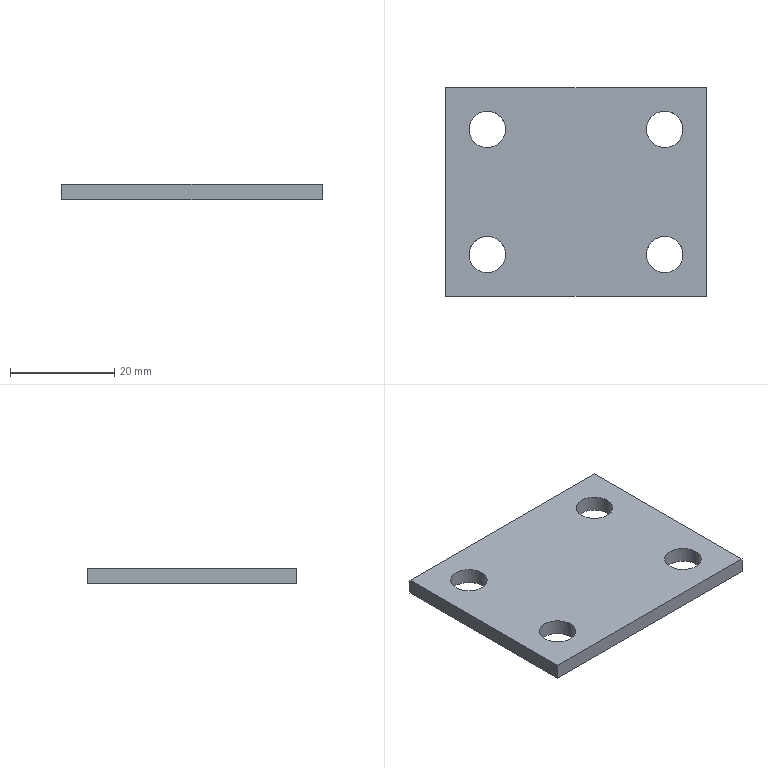Part | STEP file | Positioning_id2102_x_t | 1 solid | 14 faces | box 50 x 40 x 3 mm | volume 5538 mm3 | cylinder 8 | plane 6 | commonest cylinder face diameters 7 x8
STEP:
#1=CARTESIAN_POINT('',(0.,0.,0.));
#2=DIRECTION('',(0.,0.,1.));
#3=DIRECTION('',(1.,0.,0.));
#4=AXIS2_PLACEMENT_3D('',#1,#2,#3);
#5=CARTESIAN_POINT('',(-816.502,12.,379.5));
#6=VERTEX_POINT('',#5);
#7=CARTESIAN_POINT('',(-823.502,12.,379.5));
#8=VERTEX_POINT('',#7);
#9=CARTESIAN_POINT('',(-820.002,12.,379.5));
#10=DIRECTION('',(0.,0.,-1.));
#11=DIRECTION('',(1.,0.,0.));
#12=AXIS2_PLACEMENT_3D('',#9,#10,#11);
#13=CIRCLE('',#12,3.5);
#14=CARTESIAN_POINT('',(-773.002,-20.,379.5));
#15=DIRECTION('',(0.,0.,-1.));
#16=DIRECTION('',(-1.,0.,0.));
#17=AXIS2_PLACEMENT_3D('',#14,#15,#16);
#18=PLANE('',#17);
#19=CARTESIAN_POINT('',(47.,32.));
#20=DIRECTION('',(-1.,0.));
#21=AXIS2_PLACEMENT_2D('',#19,#20);
#22=CIRCLE('',#21,3.5);
#23=(GEOMETRIC_REPRESENTATION_CONTEXT(2)PARAMETRIC_REPRESENTATION_CONTEXT()REPRESENTATION_CONTEXT('',''));
#24=DEFINITIONAL_REPRESENTATION('',(#22),#23);
#25=PCURVE('',#18,#24);
#26=CARTESIAN_POINT('',(-820.002,12.,392.15));
#27=DIRECTION('',(0.,0.,1.));
#28=DIRECTION('',(-1.,0.,0.));
#29=AXIS2_PLACEMENT_3D('',#26,#27,#28);
#30=CYLINDRICAL_SURFACE('',#29,3.5);
#31=CARTESIAN_POINT('',(3.142,-12.65));
#32=DIRECTION('',(-1.,0.));
#33=VECTOR('',#32,1.);
#34=LINE('',#31,#33);
#35=(GEOMETRIC_REPRESENTATION_CONTEXT(2)PARAMETRIC_REPRESENTATION_CONTEXT()REPRESENTATION_CONTEXT('',''));
#36=DEFINITIONAL_REPRESENTATION('',(#34),#35);
#37=PCURVE('',#30,#36);
#38=SURFACE_CURVE('',#13,(#25,#37),.PCURVE_S1.);
#39=EDGE_CURVE('',#6,#8,#38,.T.);
#40=ORIENTED_EDGE('',*,*,#39,.T.);
#41=CARTESIAN_POINT('',(-820.002,15.5,379.5));
#42=VERTEX_POINT('',#41);
#43=CARTESIAN_POINT('',(-820.002,12.,379.5));
#44=DIRECTION('',(0.,0.,-1.));
#45=DIRECTION('',(-1.,0.,0.));
#46=AXIS2_PLACEMENT_3D('',#43,#44,#45);
#47=CIRCLE('',#46,3.5);
#48=CARTESIAN_POINT('',(47.,32.));
#49=DIRECTION('',(1.,0.));
#50=AXIS2_PLACEMENT_2D('',#48,#49);
#51=CIRCLE('',#50,3.5);
#52=(GEOMETRIC_REPRESENTATION_CONTEXT(2)PARAMETRIC_REPRESENTATION_CONTEXT()REPRESENTATION_CONTEXT('',''));
#53=DEFINITIONAL_REPRESENTATION('',(#51),#52);
#54=PCURVE('',#18,#53);
#55=CARTESIAN_POINT('',(-820.002,12.,392.15));
#56=DIRECTION('',(0.,0.,1.));
#57=DIRECTION('',(-1.,0.,0.));
#58=AXIS2_PLACEMENT_3D('',#55,#56,#57);
#59=CYLINDRICAL_SURFACE('',#58,3.5);
#60=CARTESIAN_POINT('',(6.283,-12.65));
#61=DIRECTION('',(-1.,0.));
#62=VECTOR('',#61,1.);
#63=LINE('',#60,#62);
#64=(GEOMETRIC_REPRESENTATION_CONTEXT(2)PARAMETRIC_REPRESENTATION_CONTEXT()REPRESENTATION_CONTEXT('',''));
#65=DEFINITIONAL_REPRESENTATION('',(#63),#64);
#66=PCURVE('',#59,#65);
#67=SURFACE_CURVE('',#47,(#54,#66),.PCURVE_S1.);
#68=EDGE_CURVE('',#8,#42,#67,.T.);
#69=ORIENTED_EDGE('',*,*,#68,.T.);
#70=CARTESIAN_POINT('',(-820.002,12.,379.5));
#71=DIRECTION('',(0.,0.,-1.));
#72=DIRECTION('',(0.,1.,0.));
#73=AXIS2_PLACEMENT_3D('',#70,#71,#72);
#74=CIRCLE('',#73,3.5);
#75=CARTESIAN_POINT('',(47.,32.));
#76=DIRECTION('',(0.,1.));
#77=AXIS2_PLACEMENT_2D('',#75,#76);
#78=CIRCLE('',#77,3.5);
#79=(GEOMETRIC_REPRESENTATION_CONTEXT(2)PARAMETRIC_REPRESENTATION_CONTEXT()REPRESENTATION_CONTEXT('',''));
#80=DEFINITIONAL_REPRESENTATION('',(#78),#79);
#81=PCURVE('',#18,#80);
#82=CARTESIAN_POINT('',(4.712,-12.65));
#83=DIRECTION('',(-1.,0.));
#84=VECTOR('',#83,1.);
#85=LINE('',#82,#84);
#86=(GEOMETRIC_REPRESENTATION_CONTEXT(2)PARAMETRIC_REPRESENTATION_CONTEXT()REPRESENTATION_CONTEXT('',''));
#87=DEFINITIONAL_REPRESENTATION('',(#85),#86);
#88=PCURVE('',#59,#87);
#89=SURFACE_CURVE('',#74,(#81,#88),.PCURVE_S1.);
#90=EDGE_CURVE('',#42,#6,#89,.T.);
#91=ORIENTED_EDGE('',*,*,#90,.T.);
#92=EDGE_LOOP('',(#40,#69,#91));
#93=FACE_BOUND('',#92,.T.);
#94=CARTESIAN_POINT('',(-782.502,-12.,379.5));
#95=VERTEX_POINT('',#94);
#96=CARTESIAN_POINT('',(-789.502,-12.,379.5));
#97=VERTEX_POINT('',#96);
#98=CARTESIAN_POINT('',(-786.002,-12.,379.5));
#99=DIRECTION('',(0.,0.,-1.));
#100=DIRECTION('',(1.,0.,0.));
#101=AXIS2_PLACEMENT_3D('',#98,#99,#100);
#102=CIRCLE('',#101,3.5);
#103=CARTESIAN_POINT('',(13.,8.));
#104=DIRECTION('',(-1.,0.));
#105=AXIS2_PLACEMENT_2D('',#103,#104);
#106=CIRCLE('',#105,3.5);
#107=(GEOMETRIC_REPRESENTATION_CONTEXT(2)PARAMETRIC_REPRESENTATION_CONTEXT()REPRESENTATION_CONTEXT('',''));
#108=DEFINITIONAL_REPRESENTATION('',(#106),#107);
#109=PCURVE('',#18,#108);
#110=CARTESIAN_POINT('',(-786.002,-12.,392.15));
#111=DIRECTION('',(0.,0.,1.));
#112=DIRECTION('',(-1.,0.,0.));
#113=AXIS2_PLACEMENT_3D('',#110,#111,#112);
#114=CYLINDRICAL_SURFACE('',#113,3.5);
#115=CARTESIAN_POINT('',(3.142,-12.65));
#116=DIRECTION('',(-1.,0.));
#117=VECTOR('',#116,1.);
#118=LINE('',#115,#117);
#119=(GEOMETRIC_REPRESENTATION_CONTEXT(2)PARAMETRIC_REPRESENTATION_CONTEXT()REPRESENTATION_CONTEXT('',''));
#120=DEFINITIONAL_REPRESENTATION('',(#118),#119);
#121=PCURVE('',#114,#120);
#122=SURFACE_CURVE('',#102,(#109,#121),.PCURVE_S1.);
#123=EDGE_CURVE('',#95,#97,#122,.T.);
#124=ORIENTED_EDGE('',*,*,#123,.T.);
#125=CARTESIAN_POINT('',(-786.002,-8.5,379.5));
#126=VERTEX_POINT('',#125);
#127=CARTESIAN_POINT('',(-786.002,-12.,379.5));
#128=DIRECTION('',(0.,0.,-1.));
#129=DIRECTION('',(-1.,0.,0.));
#130=AXIS2_PLACEMENT_3D('',#127,#128,#129);
#131=CIRCLE('',#130,3.5);
#132=CARTESIAN_POINT('',(13.,8.));
#133=DIRECTION('',(1.,0.));
#134=AXIS2_PLACEMENT_2D('',#132,#133);
#135=CIRCLE('',#134,3.5);
#136=(GEOMETRIC_REPRESENTATION_CONTEXT(2)PARAMETRIC_REPRESENTATION_CONTEXT()REPRESENTATION_CONTEXT('',''));
#137=DEFINITIONAL_REPRESENTATION('',(#135),#136);
#138=PCURVE('',#18,#137);
#139=CARTESIAN_POINT('',(-786.002,-12.,392.15));
#140=DIRECTION('',(0.,0.,1.));
#141=DIRECTION('',(-1.,0.,0.));
#142=AXIS2_PLACEMENT_3D('',#139,#140,#141);
#143=CYLINDRICAL_SURFACE('',#142,3.5);
#144=CARTESIAN_POINT('',(6.283,-12.65));
#145=DIRECTION('',(-1.,0.));
#146=VECTOR('',#145,1.);
#147=LINE('',#144,#146);
#148=(GEOMETRIC_REPRESENTATION_CONTEXT(2)PARAMETRIC_REPRESENTATION_CONTEXT()REPRESENTATION_CONTEXT('',''));
#149=DEFINITIONAL_REPRESENTATION('',(#147),#148);
#150=PCURVE('',#143,#149);
#151=SURFACE_CURVE('',#131,(#138,#150),.PCURVE_S1.);
#152=EDGE_CURVE('',#97,#126,#151,.T.);
#153=ORIENTED_EDGE('',*,*,#152,.T.);
#154=CARTESIAN_POINT('',(-786.002,-12.,379.5));
#155=DIRECTION('',(0.,0.,-1.));
#156=DIRECTION('',(0.,1.,0.));
#157=AXIS2_PLACEMENT_3D('',#154,#155,#156);
#158=CIRCLE('',#157,3.5);
#159=CARTESIAN_POINT('',(13.,8.));
#160=DIRECTION('',(0.,1.));
#161=AXIS2_PLACEMENT_2D('',#159,#160);
#162=CIRCLE('',#161,3.5);
#163=(GEOMETRIC_REPRESENTATION_CONTEXT(2)PARAMETRIC_REPRESENTATION_CONTEXT()REPRESENTATION_CONTEXT('',''));
#164=DEFINITIONAL_REPRESENTATION('',(#162),#163);
#165=PCURVE('',#18,#164);
#166=CARTESIAN_POINT('',(4.712,-12.65));
#167=DIRECTION('',(-1.,0.));
#168=VECTOR('',#167,1.);
#169=LINE('',#166,#168);
#170=(GEOMETRIC_REPRESENTATION_CONTEXT(2)PARAMETRIC_REPRESENTATION_CONTEXT()REPRESENTATION_CONTEXT('',''));
#171=DEFINITIONAL_REPRESENTATION('',(#169),#170);
#172=PCURVE('',#143,#171);
#173=SURFACE_CURVE('',#158,(#165,#172),.PCURVE_S1.);
#174=EDGE_CURVE('',#126,#95,#173,.T.);
#175=ORIENTED_EDGE('',*,*,#174,.T.);
#176=EDGE_LOOP('',(#124,#153,#175));
#177=FACE_BOUND('',#176,.T.);
#178=CARTESIAN_POINT('',(-782.502,12.,379.5));
#179=VERTEX_POINT('',#178);
#180=CARTESIAN_POINT('',(-789.502,12.,379.5));
#181=VERTEX_POINT('',#180);
#182=CARTESIAN_POINT('',(-786.002,12.,379.5));
#183=DIRECTION('',(0.,0.,-1.));
#184=DIRECTION('',(1.,0.,0.));
#185=AXIS2_PLACEMENT_3D('',#182,#183,#184);
#186=CIRCLE('',#185,3.5);
#187=CARTESIAN_POINT('',(13.,32.));
#188=DIRECTION('',(-1.,0.));
#189=AXIS2_PLACEMENT_2D('',#187,#188);
#190=CIRCLE('',#189,3.5);
#191=(GEOMETRIC_REPRESENTATION_CONTEXT(2)PARAMETRIC_REPRESENTATION_CONTEXT()REPRESENTATION_CONTEXT('',''));
#192=DEFINITIONAL_REPRESENTATION('',(#190),#191);
#193=PCURVE('',#18,#192);
#194=CARTESIAN_POINT('',(-786.002,12.,392.15));
#195=DIRECTION('',(0.,0.,1.));
#196=DIRECTION('',(-1.,0.,0.));
#197=AXIS2_PLACEMENT_3D('',#194,#195,#196);
#198=CYLINDRICAL_SURFACE('',#197,3.5);
#199=CARTESIAN_POINT('',(3.142,-12.65));
#200=DIRECTION('',(-1.,0.));
#201=VECTOR('',#200,1.);
#202=LINE('',#199,#201);
#203=(GEOMETRIC_REPRESENTATION_CONTEXT(2)PARAMETRIC_REPRESENTATION_CONTEXT()REPRESENTATION_CONTEXT('',''));
#204=DEFINITIONAL_REPRESENTATION('',(#202),#203);
#205=PCURVE('',#198,#204);
#206=SURFACE_CURVE('',#186,(#193,#205),.PCURVE_S1.);
#207=EDGE_CURVE('',#179,#181,#206,.T.);
#208=ORIENTED_EDGE('',*,*,#207,.T.);
#209=CARTESIAN_POINT('',(-786.002,15.5,379.5));
#210=VERTEX_POINT('',#209);
#211=CARTESIAN_POINT('',(-786.002,12.,379.5));
#212=DIRECTION('',(0.,0.,-1.));
#213=DIRECTION('',(-1.,0.,0.));
#214=AXIS2_PLACEMENT_3D('',#211,#212,#213);
#215=CIRCLE('',#214,3.5);
#216=CARTESIAN_POINT('',(13.,32.));
#217=DIRECTION('',(1.,0.));
#218=AXIS2_PLACEMENT_2D('',#216,#217);
#219=CIRCLE('',#218,3.5);
#220=(GEOMETRIC_REPRESENTATION_CONTEXT(2)PARAMETRIC_REPRESENTATION_CONTEXT()REPRESENTATION_CONTEXT('',''));
#221=DEFINITIONAL_REPRESENTATION('',(#219),#220);
#222=PCURVE('',#18,#221);
#223=CARTESIAN_POINT('',(-786.002,12.,392.15));
#224=DIRECTION('',(0.,0.,1.));
#225=DIRECTION('',(-1.,0.,0.));
#226=AXIS2_PLACEMENT_3D('',#223,#224,#225);
#227=CYLINDRICAL_SURFACE('',#226,3.5);
#228=CARTESIAN_POINT('',(6.283,-12.65));
#229=DIRECTION('',(-1.,0.));
#230=VECTOR('',#229,1.);
#231=LINE('',#228,#230);
#232=(GEOMETRIC_REPRESENTATION_CONTEXT(2)PARAMETRIC_REPRESENTATION_CONTEXT()REPRESENTATION_CONTEXT('',''));
#233=DEFINITIONAL_REPRESENTATION('',(#231),#232);
#234=PCURVE('',#227,#233);
#235=SURFACE_CURVE('',#215,(#222,#234),.PCURVE_S1.);
#236=EDGE_CURVE('',#181,#210,#235,.T.);
#237=ORIENTED_EDGE('',*,*,#236,.T.);
#238=CARTESIAN_POINT('',(-786.002,12.,379.5));
#239=DIRECTION('',(0.,0.,-1.));
#240=DIRECTION('',(0.,1.,0.));
#241=AXIS2_PLACEMENT_3D('',#238,#239,#240);
#242=CIRCLE('',#241,3.5);
#243=CARTESIAN_POINT('',(13.,32.));
#244=DIRECTION('',(0.,1.));
#245=AXIS2_PLACEMENT_2D('',#243,#244);
#246=CIRCLE('',#245,3.5);
#247=(GEOMETRIC_REPRESENTATION_CONTEXT(2)PARAMETRIC_REPRESENTATION_CONTEXT()REPRESENTATION_CONTEXT('',''));
#248=DEFINITIONAL_REPRESENTATION('',(#246),#247);
#249=PCURVE('',#18,#248);
#250=CARTESIAN_POINT('',(4.712,-12.65));
#251=DIRECTION('',(-1.,0.));
#252=VECTOR('',#251,1.);
#253=LINE('',#250,#252);
#254=(GEOMETRIC_REPRESENTATION_CONTEXT(2)PARAMETRIC_REPRESENTATION_CONTEXT()REPRESENTATION_CONTEXT('',''));
#255=DEFINITIONAL_REPRESENTATION('',(#253),#254);
#256=PCURVE('',#227,#255);
#257=SURFACE_CURVE('',#242,(#249,#256),.PCURVE_S1.);
#258=EDGE_CURVE('',#210,#179,#257,.T.);
#259=ORIENTED_EDGE('',*,*,#258,.T.);
#260=EDGE_LOOP('',(#208,#237,#259));
#261=FACE_BOUND('',#260,.T.);
#262=CARTESIAN_POINT('',(-816.502,-12.,379.5));
#263=VERTEX_POINT('',#262);
#264=CARTESIAN_POINT('',(-823.502,-12.,379.5));
#265=VERTEX_POINT('',#264);
#266=CARTESIAN_POINT('',(-820.002,-12.,379.5));
#267=DIRECTION('',(0.,0.,-1.));
#268=DIRECTION('',(1.,0.,0.));
#269=AXIS2_PLACEMENT_3D('',#266,#267,#268);
#270=CIRCLE('',#269,3.5);
#271=CARTESIAN_POINT('',(47.,8.));
#272=DIRECTION('',(-1.,0.));
#273=AXIS2_PLACEMENT_2D('',#271,#272);
#274=CIRCLE('',#273,3.5);
#275=(GEOMETRIC_REPRESENTATION_CONTEXT(2)PARAMETRIC_REPRESENTATION_CONTEXT()REPRESENTATION_CONTEXT('',''));
#276=DEFINITIONAL_REPRESENTATION('',(#274),#275);
#277=PCURVE('',#18,#276);
#278=CARTESIAN_POINT('',(-820.002,-12.,392.15));
#279=DIRECTION('',(0.,0.,1.));
#280=DIRECTION('',(-1.,0.,0.));
#281=AXIS2_PLACEMENT_3D('',#278,#279,#280);
#282=CYLINDRICAL_SURFACE('',#281,3.5);
#283=CARTESIAN_POINT('',(3.142,-12.65));
#284=DIRECTION('',(-1.,0.));
#285=VECTOR('',#284,1.);
#286=LINE('',#283,#285);
#287=(GEOMETRIC_REPRESENTATION_CONTEXT(2)PARAMETRIC_REPRESENTATION_CONTEXT()REPRESENTATION_CONTEXT('',''));
#288=DEFINITIONAL_REPRESENTATION('',(#286),#287);
#289=PCURVE('',#282,#288);
#290=SURFACE_CURVE('',#270,(#277,#289),.PCURVE_S1.);
#291=EDGE_CURVE('',#263,#265,#290,.T.);
#292=ORIENTED_EDGE('',*,*,#291,.T.);
#293=CARTESIAN_POINT('',(-820.002,-8.5,379.5));
#294=VERTEX_POINT('',#293);
#295=CARTESIAN_POINT('',(-820.002,-12.,379.5));
#296=DIRECTION('',(0.,0.,-1.));
#297=DIRECTION('',(-1.,0.,0.));
#298=AXIS2_PLACEMENT_3D('',#295,#296,#297);
#299=CIRCLE('',#298,3.5);
#300=CARTESIAN_POINT('',(47.,8.));
#301=DIRECTION('',(1.,0.));
#302=AXIS2_PLACEMENT_2D('',#300,#301);
#303=CIRCLE('',#302,3.5);
#304=(GEOMETRIC_REPRESENTATION_CONTEXT(2)PARAMETRIC_REPRESENTATION_CONTEXT()REPRESENTATION_CONTEXT('',''));
#305=DEFINITIONAL_REPRESENTATION('',(#303),#304);
#306=PCURVE('',#18,#305);
#307=CARTESIAN_POINT('',(-820.002,-12.,392.15));
#308=DIRECTION('',(0.,0.,1.));
#309=DIRECTION('',(-1.,0.,0.));
#310=AXIS2_PLACEMENT_3D('',#307,#308,#309);
#311=CYLINDRICAL_SURFACE('',#310,3.5);
#312=CARTESIAN_POINT('',(6.283,-12.65));
#313=DIRECTION('',(-1.,0.));
#314=VECTOR('',#313,1.);
#315=LINE('',#312,#314);
#316=(GEOMETRIC_REPRESENTATION_CONTEXT(2)PARAMETRIC_REPRESENTATION_CONTEXT()REPRESENTATION_CONTEXT('',''));
#317=DEFINITIONAL_REPRESENTATION('',(#315),#316);
#318=PCURVE('',#311,#317);
#319=SURFACE_CURVE('',#299,(#306,#318),.PCURVE_S1.);
#320=EDGE_CURVE('',#265,#294,#319,.T.);
#321=ORIENTED_EDGE('',*,*,#320,.T.);
#322=CARTESIAN_POINT('',(-820.002,-12.,379.5));
#323=DIRECTION('',(0.,0.,-1.));
#324=DIRECTION('',(0.,1.,0.));
#325=AXIS2_PLACEMENT_3D('',#322,#323,#324);
#326=CIRCLE('',#325,3.5);
#327=CARTESIAN_POINT('',(47.,8.));
#328=DIRECTION('',(0.,1.));
#329=AXIS2_PLACEMENT_2D('',#327,#328);
#330=CIRCLE('',#329,3.5);
#331=(GEOMETRIC_REPRESENTATION_CONTEXT(2)PARAMETRIC_REPRESENTATION_CONTEXT()REPRESENTATION_CONTEXT('',''));
#332=DEFINITIONAL_REPRESENTATION('',(#330),#331);
#333=PCURVE('',#18,#332);
#334=CARTESIAN_POINT('',(4.712,-12.65));
#335=DIRECTION('',(-1.,0.));
#336=VECTOR('',#335,1.);
#337=LINE('',#334,#336);
#338=(GEOMETRIC_REPRESENTATION_CONTEXT(2)PARAMETRIC_REPRESENTATION_CONTEXT()REPRESENTATION_CONTEXT('',''));
#339=DEFINITIONAL_REPRESENTATION('',(#337),#338);
#340=PCURVE('',#311,#339);
#341=SURFACE_CURVE('',#326,(#333,#340),.PCURVE_S1.);
#342=EDGE_CURVE('',#294,#263,#341,.T.);
#343=ORIENTED_EDGE('',*,*,#342,.T.);
#344=EDGE_LOOP('',(#292,#321,#343));
#345=FACE_BOUND('',#344,.T.);
#346=CARTESIAN_POINT('',(-828.002,20.,379.5));
#347=VERTEX_POINT('',#346);
#348=CARTESIAN_POINT('',(-778.002,20.,379.5));
#349=VERTEX_POINT('',#348);
#350=CARTESIAN_POINT('',(-828.002,20.,379.5));
#351=DIRECTION('',(1.,0.,0.));
#352=VECTOR('',#351,1.);
#353=LINE('',#350,#352);
#354=CARTESIAN_POINT('',(55.,40.));
#355=DIRECTION('',(-1.,0.));
#356=VECTOR('',#355,1.);
#357=LINE('',#354,#356);
#358=(GEOMETRIC_REPRESENTATION_CONTEXT(2)PARAMETRIC_REPRESENTATION_CONTEXT()REPRESENTATION_CONTEXT('',''));
#359=DEFINITIONAL_REPRESENTATION('',(#357),#358);
#360=PCURVE('',#18,#359);
#361=CARTESIAN_POINT('',(-826.775,20.,343.15));
#362=DIRECTION('',(0.,1.,0.));
#363=DIRECTION('',(0.,0.,1.));
#364=AXIS2_PLACEMENT_3D('',#361,#362,#363);
#365=PLANE('',#364);
#366=CARTESIAN_POINT('',(36.35,-1.227));
#367=DIRECTION('',(0.,1.));
#368=VECTOR('',#367,1.);
#369=LINE('',#366,#368);
#370=(GEOMETRIC_REPRESENTATION_CONTEXT(2)PARAMETRIC_REPRESENTATION_CONTEXT()REPRESENTATION_CONTEXT('',''));
#371=DEFINITIONAL_REPRESENTATION('',(#369),#370);
#372=PCURVE('',#365,#371);
#373=SURFACE_CURVE('',#353,(#360,#372),.PCURVE_S1.);
#374=EDGE_CURVE('',#347,#349,#373,.T.);
#375=ORIENTED_EDGE('',*,*,#374,.F.);
#376=CARTESIAN_POINT('',(-828.002,-20.,379.5));
#377=VERTEX_POINT('',#376);
#378=CARTESIAN_POINT('',(-828.002,20.,379.5));
#379=DIRECTION('',(0.,-1.,0.));
#380=VECTOR('',#379,1.);
#381=LINE('',#378,#380);
#382=CARTESIAN_POINT('',(55.,40.));
#383=DIRECTION('',(0.,-1.));
#384=VECTOR('',#383,1.);
#385=LINE('',#382,#384);
#386=(GEOMETRIC_REPRESENTATION_CONTEXT(2)PARAMETRIC_REPRESENTATION_CONTEXT()REPRESENTATION_CONTEXT('',''));
#387=DEFINITIONAL_REPRESENTATION('',(#385),#386);
#388=PCURVE('',#18,#387);
#389=CARTESIAN_POINT('',(-828.002,-20.,372.15));
#390=DIRECTION('',(1.,0.,0.));
#391=DIRECTION('',(0.,0.,-1.));
#392=AXIS2_PLACEMENT_3D('',#389,#390,#391);
#393=PLANE('',#392);
#394=CARTESIAN_POINT('',(-7.35,40.));
#395=DIRECTION('',(0.,-1.));
#396=VECTOR('',#395,1.);
#397=LINE('',#394,#396);
#398=(GEOMETRIC_REPRESENTATION_CONTEXT(2)PARAMETRIC_REPRESENTATION_CONTEXT()REPRESENTATION_CONTEXT('',''));
#399=DEFINITIONAL_REPRESENTATION('',(#397),#398);
#400=PCURVE('',#393,#399);
#401=SURFACE_CURVE('',#381,(#388,#400),.PCURVE_S1.);
#402=EDGE_CURVE('',#347,#377,#401,.T.);
#403=ORIENTED_EDGE('',*,*,#402,.T.);
#404=CARTESIAN_POINT('',(-778.002,-20.,379.5));
#405=VERTEX_POINT('',#404);
#406=CARTESIAN_POINT('',(-778.002,-20.,379.5));
#407=DIRECTION('',(-1.,0.,0.));
#408=VECTOR('',#407,1.);
#409=LINE('',#406,#408);
#410=CARTESIAN_POINT('',(5.,0.));
#411=DIRECTION('',(1.,0.));
#412=VECTOR('',#411,1.);
#413=LINE('',#410,#412);
#414=(GEOMETRIC_REPRESENTATION_CONTEXT(2)PARAMETRIC_REPRESENTATION_CONTEXT()REPRESENTATION_CONTEXT('',''));
#415=DEFINITIONAL_REPRESENTATION('',(#413),#414);
#416=PCURVE('',#18,#415);
#417=CARTESIAN_POINT('',(-826.775,-20.,343.15));
#418=DIRECTION('',(0.,-1.,0.));
#419=DIRECTION('',(0.,0.,-1.));
#420=AXIS2_PLACEMENT_3D('',#417,#418,#419);
#421=PLANE('',#420);
#422=CARTESIAN_POINT('',(-36.35,48.773));
#423=DIRECTION('',(0.,-1.));
#424=VECTOR('',#423,1.);
#425=LINE('',#422,#424);
#426=(GEOMETRIC_REPRESENTATION_CONTEXT(2)PARAMETRIC_REPRESENTATION_CONTEXT()REPRESENTATION_CONTEXT('',''));
#427=DEFINITIONAL_REPRESENTATION('',(#425),#426);
#428=PCURVE('',#421,#427);
#429=SURFACE_CURVE('',#409,(#416,#428),.PCURVE_S1.);
#430=EDGE_CURVE('',#405,#377,#429,.T.);
#431=ORIENTED_EDGE('',*,*,#430,.F.);
#432=CARTESIAN_POINT('',(-778.002,20.,379.5));
#433=DIRECTION('',(0.,-1.,0.));
#434=VECTOR('',#433,1.);
#435=LINE('',#432,#434);
#436=CARTESIAN_POINT('',(5.,40.));
#437=DIRECTION('',(0.,-1.));
#438=VECTOR('',#437,1.);
#439=LINE('',#436,#438);
#440=(GEOMETRIC_REPRESENTATION_CONTEXT(2)PARAMETRIC_REPRESENTATION_CONTEXT()REPRESENTATION_CONTEXT('',''));
#441=DEFINITIONAL_REPRESENTATION('',(#439),#440);
#442=PCURVE('',#18,#441);
#443=CARTESIAN_POINT('',(-778.002,-20.,372.15));
#444=DIRECTION('',(1.,0.,0.));
#445=DIRECTION('',(0.,0.,-1.));
#446=AXIS2_PLACEMENT_3D('',#443,#444,#445);
#447=PLANE('',#446);
#448=CARTESIAN_POINT('',(-7.35,40.));
#449=DIRECTION('',(0.,-1.));
#450=VECTOR('',#449,1.);
#451=LINE('',#448,#450);
#452=(GEOMETRIC_REPRESENTATION_CONTEXT(2)PARAMETRIC_REPRESENTATION_CONTEXT()REPRESENTATION_CONTEXT('',''));
#453=DEFINITIONAL_REPRESENTATION('',(#451),#452);
#454=PCURVE('',#447,#453);
#455=SURFACE_CURVE('',#435,(#442,#454),.PCURVE_S1.);
#456=EDGE_CURVE('',#349,#405,#455,.T.);
#457=ORIENTED_EDGE('',*,*,#456,.F.);
#458=EDGE_LOOP('',(#375,#403,#431,#457));
#459=FACE_BOUND('',#458,.T.);
#460=ADVANCED_FACE('',(#93,#177,#261,#345,#459),#18,.F.);
#461=ORIENTED_EDGE('',*,*,#456,.T.);
#462=CARTESIAN_POINT('',(-778.002,-20.,376.5));
#463=VERTEX_POINT('',#462);
#464=CARTESIAN_POINT('',(-778.002,-20.,379.5));
#465=DIRECTION('',(0.,0.,-1.));
#466=VECTOR('',#465,1.);
#467=LINE('',#464,#466);
#468=CARTESIAN_POINT('',(-7.35,0.));
#469=DIRECTION('',(1.,0.));
#470=VECTOR('',#469,1.);
#471=LINE('',#468,#470);
#472=(GEOMETRIC_REPRESENTATION_CONTEXT(2)PARAMETRIC_REPRESENTATION_CONTEXT()REPRESENTATION_CONTEXT('',''));
#473=DEFINITIONAL_REPRESENTATION('',(#471),#472);
#474=PCURVE('',#447,#473);
#475=CARTESIAN_POINT('',(-36.35,48.773));
#476=DIRECTION('',(1.,0.));
#477=VECTOR('',#476,1.);
#478=LINE('',#475,#477);
#479=(GEOMETRIC_REPRESENTATION_CONTEXT(2)PARAMETRIC_REPRESENTATION_CONTEXT()REPRESENTATION_CONTEXT('',''));
#480=DEFINITIONAL_REPRESENTATION('',(#478),#479);
#481=PCURVE('',#421,#480);
#482=SURFACE_CURVE('',#467,(#474,#481),.PCURVE_S1.);
#483=EDGE_CURVE('',#405,#463,#482,.T.);
#484=ORIENTED_EDGE('',*,*,#483,.T.);
#485=CARTESIAN_POINT('',(-778.002,20.,376.5));
#486=VERTEX_POINT('',#485);
#487=CARTESIAN_POINT('',(-778.002,-20.,376.5));
#488=DIRECTION('',(0.,1.,0.));
#489=VECTOR('',#488,1.);
#490=LINE('',#487,#489);
#491=CARTESIAN_POINT('',(-4.35,0.));
#492=DIRECTION('',(0.,1.));
#493=VECTOR('',#492,1.);
#494=LINE('',#491,#493);
#495=(GEOMETRIC_REPRESENTATION_CONTEXT(2)PARAMETRIC_REPRESENTATION_CONTEXT()REPRESENTATION_CONTEXT('',''));
#496=DEFINITIONAL_REPRESENTATION('',(#494),#495);
#497=PCURVE('',#447,#496);
#498=CARTESIAN_POINT('',(-776.775,20.,376.5));
#499=DIRECTION('',(0.,0.,-1.));
#500=DIRECTION('',(-1.,0.,0.));
#501=AXIS2_PLACEMENT_3D('',#498,#499,#500);
#502=PLANE('',#501);
#503=CARTESIAN_POINT('',(1.227,-40.));
#504=DIRECTION('',(0.,1.));
#505=VECTOR('',#504,1.);
#506=LINE('',#503,#505);
#507=(GEOMETRIC_REPRESENTATION_CONTEXT(2)PARAMETRIC_REPRESENTATION_CONTEXT()REPRESENTATION_CONTEXT('',''));
#508=DEFINITIONAL_REPRESENTATION('',(#506),#507);
#509=PCURVE('',#502,#508);
#510=SURFACE_CURVE('',#490,(#497,#509),.PCURVE_S1.);
#511=EDGE_CURVE('',#463,#486,#510,.T.);
#512=ORIENTED_EDGE('',*,*,#511,.T.);
#513=CARTESIAN_POINT('',(-778.002,20.,376.5));
#514=DIRECTION('',(0.,0.,1.));
#515=VECTOR('',#514,1.);
#516=LINE('',#513,#515);
#517=CARTESIAN_POINT('',(-4.35,40.));
#518=DIRECTION('',(-1.,0.));
#519=VECTOR('',#518,1.);
#520=LINE('',#517,#519);
#521=(GEOMETRIC_REPRESENTATION_CONTEXT(2)PARAMETRIC_REPRESENTATION_CONTEXT()REPRESENTATION_CONTEXT('',''));
#522=DEFINITIONAL_REPRESENTATION('',(#520),#521);
#523=PCURVE('',#447,#522);
#524=CARTESIAN_POINT('',(33.35,48.773));
#525=DIRECTION('',(1.,0.));
#526=VECTOR('',#525,1.);
#527=LINE('',#524,#526);
#528=(GEOMETRIC_REPRESENTATION_CONTEXT(2)PARAMETRIC_REPRESENTATION_CONTEXT()REPRESENTATION_CONTEXT('',''));
#529=DEFINITIONAL_REPRESENTATION('',(#527),#528);
#530=PCURVE('',#365,#529);
#531=SURFACE_CURVE('',#516,(#523,#530),.PCURVE_S1.);
#532=EDGE_CURVE('',#486,#349,#531,.T.);
#533=ORIENTED_EDGE('',*,*,#532,.T.);
#534=EDGE_LOOP('',(#461,#484,#512,#533));
#535=FACE_BOUND('',#534,.T.);
#536=ADVANCED_FACE('',(#535),#447,.T.);
#537=CARTESIAN_POINT('',(-789.502,12.,376.5));
#538=VERTEX_POINT('',#537);
#539=CARTESIAN_POINT('',(-782.502,12.,376.5));
#540=VERTEX_POINT('',#539);
#541=CARTESIAN_POINT('',(-786.002,12.,376.5));
#542=DIRECTION('',(0.,0.,1.));
#543=DIRECTION('',(1.,0.,0.));
#544=AXIS2_PLACEMENT_3D('',#541,#542,#543);
#545=CIRCLE('',#544,3.5);
#546=CARTESIAN_POINT('',(-3.142,-15.65));
#547=DIRECTION('',(1.,0.));
#548=VECTOR('',#547,1.);
#549=LINE('',#546,#548);
#550=(GEOMETRIC_REPRESENTATION_CONTEXT(2)PARAMETRIC_REPRESENTATION_CONTEXT()REPRESENTATION_CONTEXT('',''));
#551=DEFINITIONAL_REPRESENTATION('',(#549),#550);
#552=PCURVE('',#198,#551);
#553=CARTESIAN_POINT('',(5.727,-8.));
#554=CARTESIAN_POINT('',(5.727,-1.938));
#555=CARTESIAN_POINT('',(10.977,-4.969));
#556=CARTESIAN_POINT('',(16.227,-8.));
#557=CARTESIAN_POINT('',(10.977,-11.031));
#558=CARTESIAN_POINT('',(5.727,-14.062));
#559=CARTESIAN_POINT('',(5.727,-8.));
#560=(BOUNDED_CURVE()B_SPLINE_CURVE(2,(#553,#554,#555,#556,#557,#558,#559),.UNSPECIFIED.,.T.,.F.)B_SPLINE_CURVE_WITH_KNOTS((1,2,2,2,2,1),(-2.094,0.,2.094,4.189,6.283,8.378),.UNSPECIFIED.)CURVE()GEOMETRIC_REPRESENTATION_ITEM()RATIONAL_B_SPLINE_CURVE((1.,0.5,1.,0.5,1.,0.5,1.))REPRESENTATION_ITEM(''));
#561=(GEOMETRIC_REPRESENTATION_CONTEXT(2)PARAMETRIC_REPRESENTATION_CONTEXT()REPRESENTATION_CONTEXT('',''));
#562=DEFINITIONAL_REPRESENTATION('',(#560),#561);
#563=PCURVE('',#502,#562);
#564=SURFACE_CURVE('',#545,(#552,#563),.PCURVE_S1.);
#565=EDGE_CURVE('',#538,#540,#564,.T.);
#566=ORIENTED_EDGE('',*,*,#565,.T.);
#567=CARTESIAN_POINT('',(-782.502,12.,379.5));
#568=DIRECTION('',(0.,0.,-1.));
#569=VECTOR('',#568,1.);
#570=LINE('',#567,#569);
#571=CARTESIAN_POINT('',(3.142,-12.65));
#572=DIRECTION('',(0.,-1.));
#573=VECTOR('',#572,1.);
#574=LINE('',#571,#573);
#575=(GEOMETRIC_REPRESENTATION_CONTEXT(2)PARAMETRIC_REPRESENTATION_CONTEXT()REPRESENTATION_CONTEXT('',''));
#576=DEFINITIONAL_REPRESENTATION('',(#574),#575);
#577=PCURVE('',#198,#576);
#578=CARTESIAN_POINT('',(3.142,-12.65));
#579=DIRECTION('',(0.,-1.));
#580=VECTOR('',#579,1.);
#581=LINE('',#578,#580);
#582=(GEOMETRIC_REPRESENTATION_CONTEXT(2)PARAMETRIC_REPRESENTATION_CONTEXT()REPRESENTATION_CONTEXT('',''));
#583=DEFINITIONAL_REPRESENTATION('',(#581),#582);
#584=PCURVE('',#227,#583);
#585=SURFACE_CURVE('',#570,(#577,#584),.PCURVE_S1.);
#586=EDGE_CURVE('',#179,#540,#585,.T.);
#587=ORIENTED_EDGE('',*,*,#586,.F.);
#588=ORIENTED_EDGE('',*,*,#207,.T.);
#589=CARTESIAN_POINT('',(-789.502,12.,379.5));
#590=DIRECTION('',(0.,0.,1.));
#591=VECTOR('',#590,1.);
#592=LINE('',#589,#591);
#593=CARTESIAN_POINT('',(0.,-12.65));
#594=DIRECTION('',(0.,1.));
#595=VECTOR('',#594,1.);
#596=LINE('',#593,#595);
#597=(GEOMETRIC_REPRESENTATION_CONTEXT(2)PARAMETRIC_REPRESENTATION_CONTEXT()REPRESENTATION_CONTEXT('',''));
#598=DEFINITIONAL_REPRESENTATION('',(#596),#597);
#599=PCURVE('',#198,#598);
#600=CARTESIAN_POINT('',(6.283,-12.65));
#601=DIRECTION('',(0.,1.));
#602=VECTOR('',#601,1.);
#603=LINE('',#600,#602);
#604=(GEOMETRIC_REPRESENTATION_CONTEXT(2)PARAMETRIC_REPRESENTATION_CONTEXT()REPRESENTATION_CONTEXT('',''));
#605=DEFINITIONAL_REPRESENTATION('',(#603),#604);
#606=PCURVE('',#227,#605);
#607=SURFACE_CURVE('',#592,(#599,#606),.PCURVE_S1.);
#608=EDGE_CURVE('',#538,#181,#607,.T.);
#609=ORIENTED_EDGE('',*,*,#608,.F.);
#610=EDGE_LOOP('',(#566,#587,#588,#609));
#611=FACE_BOUND('',#610,.F.);
#612=ADVANCED_FACE('',(#611),#198,.F.);
#613=CARTESIAN_POINT('',(-789.502,-12.,376.5));
#614=VERTEX_POINT('',#613);
#615=CARTESIAN_POINT('',(-782.502,-12.,376.5));
#616=VERTEX_POINT('',#615);
#617=CARTESIAN_POINT('',(-786.002,-12.,376.5));
#618=DIRECTION('',(0.,0.,1.));
#619=DIRECTION('',(1.,0.,0.));
#620=AXIS2_PLACEMENT_3D('',#617,#618,#619);
#621=CIRCLE('',#620,3.5);
#622=CARTESIAN_POINT('',(-3.142,-15.65));
#623=DIRECTION('',(1.,0.));
#624=VECTOR('',#623,1.);
#625=LINE('',#622,#624);
#626=(GEOMETRIC_REPRESENTATION_CONTEXT(2)PARAMETRIC_REPRESENTATION_CONTEXT()REPRESENTATION_CONTEXT('',''));
#627=DEFINITIONAL_REPRESENTATION('',(#625),#626);
#628=PCURVE('',#114,#627);
#629=CARTESIAN_POINT('',(5.727,-32.));
#630=CARTESIAN_POINT('',(5.727,-25.938));
#631=CARTESIAN_POINT('',(10.977,-28.969));
#632=CARTESIAN_POINT('',(16.227,-32.));
#633=CARTESIAN_POINT('',(10.977,-35.031));
#634=CARTESIAN_POINT('',(5.727,-38.062));
#635=CARTESIAN_POINT('',(5.727,-32.));
#636=(BOUNDED_CURVE()B_SPLINE_CURVE(2,(#629,#630,#631,#632,#633,#634,#635),.UNSPECIFIED.,.T.,.F.)B_SPLINE_CURVE_WITH_KNOTS((1,2,2,2,2,1),(-2.094,0.,2.094,4.189,6.283,8.378),.UNSPECIFIED.)CURVE()GEOMETRIC_REPRESENTATION_ITEM()RATIONAL_B_SPLINE_CURVE((1.,0.5,1.,0.5,1.,0.5,1.))REPRESENTATION_ITEM(''));
#637=(GEOMETRIC_REPRESENTATION_CONTEXT(2)PARAMETRIC_REPRESENTATION_CONTEXT()REPRESENTATION_CONTEXT('',''));
#638=DEFINITIONAL_REPRESENTATION('',(#636),#637);
#639=PCURVE('',#502,#638);
#640=SURFACE_CURVE('',#621,(#628,#639),.PCURVE_S1.);
#641=EDGE_CURVE('',#614,#616,#640,.T.);
#642=ORIENTED_EDGE('',*,*,#641,.T.);
#643=CARTESIAN_POINT('',(-782.502,-12.,379.5));
#644=DIRECTION('',(0.,0.,1.));
#645=VECTOR('',#644,1.);
#646=LINE('',#643,#645);
#647=CARTESIAN_POINT('',(3.142,-12.65));
#648=DIRECTION('',(0.,1.));
#649=VECTOR('',#648,1.);
#650=LINE('',#647,#649);
#651=(GEOMETRIC_REPRESENTATION_CONTEXT(2)PARAMETRIC_REPRESENTATION_CONTEXT()REPRESENTATION_CONTEXT('',''));
#652=DEFINITIONAL_REPRESENTATION('',(#650),#651);
#653=PCURVE('',#114,#652);
#654=CARTESIAN_POINT('',(3.142,-12.65));
#655=DIRECTION('',(0.,1.));
#656=VECTOR('',#655,1.);
#657=LINE('',#654,#656);
#658=(GEOMETRIC_REPRESENTATION_CONTEXT(2)PARAMETRIC_REPRESENTATION_CONTEXT()REPRESENTATION_CONTEXT('',''));
#659=DEFINITIONAL_REPRESENTATION('',(#657),#658);
#660=PCURVE('',#143,#659);
#661=SURFACE_CURVE('',#646,(#653,#660),.PCURVE_S1.);
#662=EDGE_CURVE('',#616,#95,#661,.T.);
#663=ORIENTED_EDGE('',*,*,#662,.T.);
#664=ORIENTED_EDGE('',*,*,#123,.T.);
#665=CARTESIAN_POINT('',(-789.502,-12.,379.5));
#666=DIRECTION('',(0.,0.,-1.));
#667=VECTOR('',#666,1.);
#668=LINE('',#665,#667);
#669=CARTESIAN_POINT('',(0.,-12.65));
#670=DIRECTION('',(0.,-1.));
#671=VECTOR('',#670,1.);
#672=LINE('',#669,#671);
#673=(GEOMETRIC_REPRESENTATION_CONTEXT(2)PARAMETRIC_REPRESENTATION_CONTEXT()REPRESENTATION_CONTEXT('',''));
#674=DEFINITIONAL_REPRESENTATION('',(#672),#673);
#675=PCURVE('',#114,#674);
#676=CARTESIAN_POINT('',(6.283,-12.65));
#677=DIRECTION('',(0.,-1.));
#678=VECTOR('',#677,1.);
#679=LINE('',#676,#678);
#680=(GEOMETRIC_REPRESENTATION_CONTEXT(2)PARAMETRIC_REPRESENTATION_CONTEXT()REPRESENTATION_CONTEXT('',''));
#681=DEFINITIONAL_REPRESENTATION('',(#679),#680);
#682=PCURVE('',#143,#681);
#683=SURFACE_CURVE('',#668,(#675,#682),.PCURVE_S1.);
#684=EDGE_CURVE('',#97,#614,#683,.T.);
#685=ORIENTED_EDGE('',*,*,#684,.T.);
#686=EDGE_LOOP('',(#642,#663,#664,#685));
#687=FACE_BOUND('',#686,.F.);
#688=ADVANCED_FACE('',(#687),#114,.F.);
#689=CARTESIAN_POINT('',(-823.502,-12.,376.5));
#690=VERTEX_POINT('',#689);
#691=CARTESIAN_POINT('',(-816.502,-12.,376.5));
#692=VERTEX_POINT('',#691);
#693=CARTESIAN_POINT('',(-820.002,-12.,376.5));
#694=DIRECTION('',(0.,0.,1.));
#695=DIRECTION('',(1.,0.,0.));
#696=AXIS2_PLACEMENT_3D('',#693,#694,#695);
#697=CIRCLE('',#696,3.5);
#698=CARTESIAN_POINT('',(-3.142,-15.65));
#699=DIRECTION('',(1.,0.));
#700=VECTOR('',#699,1.);
#701=LINE('',#698,#700);
#702=(GEOMETRIC_REPRESENTATION_CONTEXT(2)PARAMETRIC_REPRESENTATION_CONTEXT()REPRESENTATION_CONTEXT('',''));
#703=DEFINITIONAL_REPRESENTATION('',(#701),#702);
#704=PCURVE('',#282,#703);
#705=CARTESIAN_POINT('',(39.727,-32.));
#706=CARTESIAN_POINT('',(39.727,-25.938));
#707=CARTESIAN_POINT('',(44.977,-28.969));
#708=CARTESIAN_POINT('',(50.227,-32.));
#709=CARTESIAN_POINT('',(44.977,-35.031));
#710=CARTESIAN_POINT('',(39.727,-38.062));
#711=CARTESIAN_POINT('',(39.727,-32.));
#712=(BOUNDED_CURVE()B_SPLINE_CURVE(2,(#705,#706,#707,#708,#709,#710,#711),.UNSPECIFIED.,.T.,.F.)B_SPLINE_CURVE_WITH_KNOTS((1,2,2,2,2,1),(-2.094,0.,2.094,4.189,6.283,8.378),.UNSPECIFIED.)CURVE()GEOMETRIC_REPRESENTATION_ITEM()RATIONAL_B_SPLINE_CURVE((1.,0.5,1.,0.5,1.,0.5,1.))REPRESENTATION_ITEM(''));
#713=(GEOMETRIC_REPRESENTATION_CONTEXT(2)PARAMETRIC_REPRESENTATION_CONTEXT()REPRESENTATION_CONTEXT('',''));
#714=DEFINITIONAL_REPRESENTATION('',(#712),#713);
#715=PCURVE('',#502,#714);
#716=SURFACE_CURVE('',#697,(#704,#715),.PCURVE_S1.);
#717=EDGE_CURVE('',#690,#692,#716,.T.);
#718=ORIENTED_EDGE('',*,*,#717,.T.);
#719=CARTESIAN_POINT('',(-816.502,-12.,379.5));
#720=DIRECTION('',(0.,0.,1.));
#721=VECTOR('',#720,1.);
#722=LINE('',#719,#721);
#723=CARTESIAN_POINT('',(3.142,-12.65));
#724=DIRECTION('',(0.,1.));
#725=VECTOR('',#724,1.);
#726=LINE('',#723,#725);
#727=(GEOMETRIC_REPRESENTATION_CONTEXT(2)PARAMETRIC_REPRESENTATION_CONTEXT()REPRESENTATION_CONTEXT('',''));
#728=DEFINITIONAL_REPRESENTATION('',(#726),#727);
#729=PCURVE('',#282,#728);
#730=CARTESIAN_POINT('',(3.142,-12.65));
#731=DIRECTION('',(0.,1.));
#732=VECTOR('',#731,1.);
#733=LINE('',#730,#732);
#734=(GEOMETRIC_REPRESENTATION_CONTEXT(2)PARAMETRIC_REPRESENTATION_CONTEXT()REPRESENTATION_CONTEXT('',''));
#735=DEFINITIONAL_REPRESENTATION('',(#733),#734);
#736=PCURVE('',#311,#735);
#737=SURFACE_CURVE('',#722,(#729,#736),.PCURVE_S1.);
#738=EDGE_CURVE('',#692,#263,#737,.T.);
#739=ORIENTED_EDGE('',*,*,#738,.T.);
#740=ORIENTED_EDGE('',*,*,#291,.T.);
#741=CARTESIAN_POINT('',(-823.502,-12.,379.5));
#742=DIRECTION('',(0.,0.,-1.));
#743=VECTOR('',#742,1.);
#744=LINE('',#741,#743);
#745=CARTESIAN_POINT('',(0.,-12.65));
#746=DIRECTION('',(0.,-1.));
#747=VECTOR('',#746,1.);
#748=LINE('',#745,#747);
#749=(GEOMETRIC_REPRESENTATION_CONTEXT(2)PARAMETRIC_REPRESENTATION_CONTEXT()REPRESENTATION_CONTEXT('',''));
#750=DEFINITIONAL_REPRESENTATION('',(#748),#749);
#751=PCURVE('',#282,#750);
#752=CARTESIAN_POINT('',(6.283,-12.65));
#753=DIRECTION('',(0.,-1.));
#754=VECTOR('',#753,1.);
#755=LINE('',#752,#754);
#756=(GEOMETRIC_REPRESENTATION_CONTEXT(2)PARAMETRIC_REPRESENTATION_CONTEXT()REPRESENTATION_CONTEXT('',''));
#757=DEFINITIONAL_REPRESENTATION('',(#755),#756);
#758=PCURVE('',#311,#757);
#759=SURFACE_CURVE('',#744,(#751,#758),.PCURVE_S1.);
#760=EDGE_CURVE('',#265,#690,#759,.T.);
#761=ORIENTED_EDGE('',*,*,#760,.T.);
#762=EDGE_LOOP('',(#718,#739,#740,#761));
#763=FACE_BOUND('',#762,.F.);
#764=ADVANCED_FACE('',(#763),#282,.F.);
#765=CARTESIAN_POINT('',(-823.502,12.,376.5));
#766=VERTEX_POINT('',#765);
#767=CARTESIAN_POINT('',(-816.502,12.,376.5));
#768=VERTEX_POINT('',#767);
#769=CARTESIAN_POINT('',(-820.002,12.,376.5));
#770=DIRECTION('',(0.,0.,1.));
#771=DIRECTION('',(1.,0.,0.));
#772=AXIS2_PLACEMENT_3D('',#769,#770,#771);
#773=CIRCLE('',#772,3.5);
#774=CARTESIAN_POINT('',(-3.142,-15.65));
#775=DIRECTION('',(1.,0.));
#776=VECTOR('',#775,1.);
#777=LINE('',#774,#776);
#778=(GEOMETRIC_REPRESENTATION_CONTEXT(2)PARAMETRIC_REPRESENTATION_CONTEXT()REPRESENTATION_CONTEXT('',''));
#779=DEFINITIONAL_REPRESENTATION('',(#777),#778);
#780=PCURVE('',#30,#779);
#781=CARTESIAN_POINT('',(39.727,-8.));
#782=CARTESIAN_POINT('',(39.727,-1.938));
#783=CARTESIAN_POINT('',(44.977,-4.969));
#784=CARTESIAN_POINT('',(50.227,-8.));
#785=CARTESIAN_POINT('',(44.977,-11.031));
#786=CARTESIAN_POINT('',(39.727,-14.062));
#787=CARTESIAN_POINT('',(39.727,-8.));
#788=(BOUNDED_CURVE()B_SPLINE_CURVE(2,(#781,#782,#783,#784,#785,#786,#787),.UNSPECIFIED.,.T.,.F.)B_SPLINE_CURVE_WITH_KNOTS((1,2,2,2,2,1),(-2.094,0.,2.094,4.189,6.283,8.378),.UNSPECIFIED.)CURVE()GEOMETRIC_REPRESENTATION_ITEM()RATIONAL_B_SPLINE_CURVE((1.,0.5,1.,0.5,1.,0.5,1.))REPRESENTATION_ITEM(''));
#789=(GEOMETRIC_REPRESENTATION_CONTEXT(2)PARAMETRIC_REPRESENTATION_CONTEXT()REPRESENTATION_CONTEXT('',''));
#790=DEFINITIONAL_REPRESENTATION('',(#788),#789);
#791=PCURVE('',#502,#790);
#792=SURFACE_CURVE('',#773,(#780,#791),.PCURVE_S1.);
#793=EDGE_CURVE('',#766,#768,#792,.T.);
#794=ORIENTED_EDGE('',*,*,#793,.T.);
#795=CARTESIAN_POINT('',(-816.502,12.,379.5));
#796=DIRECTION('',(0.,0.,-1.));
#797=VECTOR('',#796,1.);
#798=LINE('',#795,#797);
#799=CARTESIAN_POINT('',(3.142,-12.65));
#800=DIRECTION('',(0.,-1.));
#801=VECTOR('',#800,1.);
#802=LINE('',#799,#801);
#803=(GEOMETRIC_REPRESENTATION_CONTEXT(2)PARAMETRIC_REPRESENTATION_CONTEXT()REPRESENTATION_CONTEXT('',''));
#804=DEFINITIONAL_REPRESENTATION('',(#802),#803);
#805=PCURVE('',#30,#804);
#806=CARTESIAN_POINT('',(3.142,-12.65));
#807=DIRECTION('',(0.,-1.));
#808=VECTOR('',#807,1.);
#809=LINE('',#806,#808);
#810=(GEOMETRIC_REPRESENTATION_CONTEXT(2)PARAMETRIC_REPRESENTATION_CONTEXT()REPRESENTATION_CONTEXT('',''));
#811=DEFINITIONAL_REPRESENTATION('',(#809),#810);
#812=PCURVE('',#59,#811);
#813=SURFACE_CURVE('',#798,(#805,#812),.PCURVE_S1.);
#814=EDGE_CURVE('',#6,#768,#813,.T.);
#815=ORIENTED_EDGE('',*,*,#814,.F.);
#816=ORIENTED_EDGE('',*,*,#39,.T.);
#817=CARTESIAN_POINT('',(-823.502,12.,379.5));
#818=DIRECTION('',(0.,0.,1.));
#819=VECTOR('',#818,1.);
#820=LINE('',#817,#819);
#821=CARTESIAN_POINT('',(0.,-12.65));
#822=DIRECTION('',(0.,1.));
#823=VECTOR('',#822,1.);
#824=LINE('',#821,#823);
#825=(GEOMETRIC_REPRESENTATION_CONTEXT(2)PARAMETRIC_REPRESENTATION_CONTEXT()REPRESENTATION_CONTEXT('',''));
#826=DEFINITIONAL_REPRESENTATION('',(#824),#825);
#827=PCURVE('',#30,#826);
#828=CARTESIAN_POINT('',(6.283,-12.65));
#829=DIRECTION('',(0.,1.));
#830=VECTOR('',#829,1.);
#831=LINE('',#828,#830);
#832=(GEOMETRIC_REPRESENTATION_CONTEXT(2)PARAMETRIC_REPRESENTATION_CONTEXT()REPRESENTATION_CONTEXT('',''));
#833=DEFINITIONAL_REPRESENTATION('',(#831),#832);
#834=PCURVE('',#59,#833);
#835=SURFACE_CURVE('',#820,(#827,#834),.PCURVE_S1.);
#836=EDGE_CURVE('',#766,#8,#835,.T.);
#837=ORIENTED_EDGE('',*,*,#836,.F.);
#838=EDGE_LOOP('',(#794,#815,#816,#837));
#839=FACE_BOUND('',#838,.F.);
#840=ADVANCED_FACE('',(#839),#30,.F.);
#841=CARTESIAN_POINT('',(-828.002,20.,376.5));
#842=VERTEX_POINT('',#841);
#843=CARTESIAN_POINT('',(-828.002,20.,376.5));
#844=DIRECTION('',(0.,0.,1.));
#845=VECTOR('',#844,1.);
#846=LINE('',#843,#845);
#847=CARTESIAN_POINT('',(-4.35,40.));
#848=DIRECTION('',(-1.,0.));
#849=VECTOR('',#848,1.);
#850=LINE('',#847,#849);
#851=(GEOMETRIC_REPRESENTATION_CONTEXT(2)PARAMETRIC_REPRESENTATION_CONTEXT()REPRESENTATION_CONTEXT('',''));
#852=DEFINITIONAL_REPRESENTATION('',(#850),#851);
#853=PCURVE('',#393,#852);
#854=CARTESIAN_POINT('',(33.35,-1.227));
#855=DIRECTION('',(1.,0.));
#856=VECTOR('',#855,1.);
#857=LINE('',#854,#856);
#858=(GEOMETRIC_REPRESENTATION_CONTEXT(2)PARAMETRIC_REPRESENTATION_CONTEXT()REPRESENTATION_CONTEXT('',''));
#859=DEFINITIONAL_REPRESENTATION('',(#857),#858);
#860=PCURVE('',#365,#859);
#861=SURFACE_CURVE('',#846,(#853,#860),.PCURVE_S1.);
#862=EDGE_CURVE('',#842,#347,#861,.T.);
#863=ORIENTED_EDGE('',*,*,#862,.F.);
#864=CARTESIAN_POINT('',(-828.002,-20.,376.5));
#865=VERTEX_POINT('',#864);
#866=CARTESIAN_POINT('',(-828.002,-20.,376.5));
#867=DIRECTION('',(0.,1.,0.));
#868=VECTOR('',#867,1.);
#869=LINE('',#866,#868);
#870=CARTESIAN_POINT('',(-4.35,0.));
#871=DIRECTION('',(0.,1.));
#872=VECTOR('',#871,1.);
#873=LINE('',#870,#872);
#874=(GEOMETRIC_REPRESENTATION_CONTEXT(2)PARAMETRIC_REPRESENTATION_CONTEXT()REPRESENTATION_CONTEXT('',''));
#875=DEFINITIONAL_REPRESENTATION('',(#873),#874);
#876=PCURVE('',#393,#875);
#877=CARTESIAN_POINT('',(51.227,-40.));
#878=DIRECTION('',(0.,1.));
#879=VECTOR('',#878,1.);
#880=LINE('',#877,#879);
#881=(GEOMETRIC_REPRESENTATION_CONTEXT(2)PARAMETRIC_REPRESENTATION_CONTEXT()REPRESENTATION_CONTEXT('',''));
#882=DEFINITIONAL_REPRESENTATION('',(#880),#881);
#883=PCURVE('',#502,#882);
#884=SURFACE_CURVE('',#869,(#876,#883),.PCURVE_S1.);
#885=EDGE_CURVE('',#865,#842,#884,.T.);
#886=ORIENTED_EDGE('',*,*,#885,.F.);
#887=CARTESIAN_POINT('',(-828.002,-20.,379.5));
#888=DIRECTION('',(0.,0.,-1.));
#889=VECTOR('',#888,1.);
#890=LINE('',#887,#889);
#891=CARTESIAN_POINT('',(-7.35,0.));
#892=DIRECTION('',(1.,0.));
#893=VECTOR('',#892,1.);
#894=LINE('',#891,#893);
#895=(GEOMETRIC_REPRESENTATION_CONTEXT(2)PARAMETRIC_REPRESENTATION_CONTEXT()REPRESENTATION_CONTEXT('',''));
#896=DEFINITIONAL_REPRESENTATION('',(#894),#895);
#897=PCURVE('',#393,#896);
#898=CARTESIAN_POINT('',(-36.35,-1.227));
#899=DIRECTION('',(1.,0.));
#900=VECTOR('',#899,1.);
#901=LINE('',#898,#900);
#902=(GEOMETRIC_REPRESENTATION_CONTEXT(2)PARAMETRIC_REPRESENTATION_CONTEXT()REPRESENTATION_CONTEXT('',''));
#903=DEFINITIONAL_REPRESENTATION('',(#901),#902);
#904=PCURVE('',#421,#903);
#905=SURFACE_CURVE('',#890,(#897,#904),.PCURVE_S1.);
#906=EDGE_CURVE('',#377,#865,#905,.T.);
#907=ORIENTED_EDGE('',*,*,#906,.F.);
#908=ORIENTED_EDGE('',*,*,#402,.F.);
#909=EDGE_LOOP('',(#863,#886,#907,#908));
#910=FACE_BOUND('',#909,.T.);
#911=ADVANCED_FACE('',(#910),#393,.F.);
#912=ORIENTED_EDGE('',*,*,#430,.T.);
#913=ORIENTED_EDGE('',*,*,#906,.T.);
#914=CARTESIAN_POINT('',(-778.002,-20.,376.5));
#915=DIRECTION('',(-1.,0.,0.));
#916=VECTOR('',#915,1.);
#917=LINE('',#914,#916);
#918=CARTESIAN_POINT('',(-33.35,48.773));
#919=DIRECTION('',(0.,-1.));
#920=VECTOR('',#919,1.);
#921=LINE('',#918,#920);
#922=(GEOMETRIC_REPRESENTATION_CONTEXT(2)PARAMETRIC_REPRESENTATION_CONTEXT()REPRESENTATION_CONTEXT('',''));
#923=DEFINITIONAL_REPRESENTATION('',(#921),#922);
#924=PCURVE('',#421,#923);
#925=CARTESIAN_POINT('',(1.227,-40.));
#926=DIRECTION('',(1.,0.));
#927=VECTOR('',#926,1.);
#928=LINE('',#925,#927);
#929=(GEOMETRIC_REPRESENTATION_CONTEXT(2)PARAMETRIC_REPRESENTATION_CONTEXT()REPRESENTATION_CONTEXT('',''));
#930=DEFINITIONAL_REPRESENTATION('',(#928),#929);
#931=PCURVE('',#502,#930);
#932=SURFACE_CURVE('',#917,(#924,#931),.PCURVE_S1.);
#933=EDGE_CURVE('',#463,#865,#932,.T.);
#934=ORIENTED_EDGE('',*,*,#933,.F.);
#935=ORIENTED_EDGE('',*,*,#483,.F.);
#936=EDGE_LOOP('',(#912,#913,#934,#935));
#937=FACE_BOUND('',#936,.T.);
#938=ADVANCED_FACE('',(#937),#421,.T.);
#939=ORIENTED_EDGE('',*,*,#374,.T.);
#940=ORIENTED_EDGE('',*,*,#532,.F.);
#941=CARTESIAN_POINT('',(-828.002,20.,376.5));
#942=DIRECTION('',(1.,0.,0.));
#943=VECTOR('',#942,1.);
#944=LINE('',#941,#943);
#945=CARTESIAN_POINT('',(33.35,-1.227));
#946=DIRECTION('',(0.,1.));
#947=VECTOR('',#946,1.);
#948=LINE('',#945,#947);
#949=(GEOMETRIC_REPRESENTATION_CONTEXT(2)PARAMETRIC_REPRESENTATION_CONTEXT()REPRESENTATION_CONTEXT('',''));
#950=DEFINITIONAL_REPRESENTATION('',(#948),#949);
#951=PCURVE('',#365,#950);
#952=CARTESIAN_POINT('',(51.227,0.));
#953=DIRECTION('',(-1.,0.));
#954=VECTOR('',#953,1.);
#955=LINE('',#952,#954);
#956=(GEOMETRIC_REPRESENTATION_CONTEXT(2)PARAMETRIC_REPRESENTATION_CONTEXT()REPRESENTATION_CONTEXT('',''));
#957=DEFINITIONAL_REPRESENTATION('',(#955),#956);
#958=PCURVE('',#502,#957);
#959=SURFACE_CURVE('',#944,(#951,#958),.PCURVE_S1.);
#960=EDGE_CURVE('',#842,#486,#959,.T.);
#961=ORIENTED_EDGE('',*,*,#960,.F.);
#962=ORIENTED_EDGE('',*,*,#862,.T.);
#963=EDGE_LOOP('',(#939,#940,#961,#962));
#964=FACE_BOUND('',#963,.T.);
#965=ADVANCED_FACE('',(#964),#365,.T.);
#966=CARTESIAN_POINT('',(-782.502,12.,376.5));
#967=CARTESIAN_POINT('',(-782.502,15.5,376.5));
#968=CARTESIAN_POINT('',(-786.002,17.25,376.5));
#969=CARTESIAN_POINT('',(-789.502,15.5,376.5));
#970=CARTESIAN_POINT('',(-789.502,12.,376.5));
#971=(BOUNDED_CURVE()B_SPLINE_CURVE(4,(#966,#967,#968,#969,#970),.UNSPECIFIED.,.F.,.F.)B_SPLINE_CURVE_WITH_KNOTS((5,5),(0.,1.),.PIECEWISE_BEZIER_KNOTS.)CURVE()GEOMETRIC_REPRESENTATION_ITEM()RATIONAL_B_SPLINE_CURVE((1.,0.7071,0.6667,0.7071,1.))REPRESENTATION_ITEM(''));
#972=CARTESIAN_POINT('',(5.727,-8.));
#973=CARTESIAN_POINT('',(5.727,-4.5));
#974=CARTESIAN_POINT('',(9.227,-2.75));
#975=CARTESIAN_POINT('',(12.727,-4.5));
#976=CARTESIAN_POINT('',(12.727,-8.));
#977=(BOUNDED_CURVE()B_SPLINE_CURVE(4,(#972,#973,#974,#975,#976),.UNSPECIFIED.,.F.,.F.)B_SPLINE_CURVE_WITH_KNOTS((5,5),(0.,1.),.PIECEWISE_BEZIER_KNOTS.)CURVE()GEOMETRIC_REPRESENTATION_ITEM()RATIONAL_B_SPLINE_CURVE((1.,0.7071,0.6667,0.7071,1.))REPRESENTATION_ITEM(''));
#978=(GEOMETRIC_REPRESENTATION_CONTEXT(2)PARAMETRIC_REPRESENTATION_CONTEXT()REPRESENTATION_CONTEXT('',''));
#979=DEFINITIONAL_REPRESENTATION('',(#977),#978);
#980=PCURVE('',#502,#979);
#981=CARTESIAN_POINT('',(3.142,-15.65));
#982=CARTESIAN_POINT('',(3.184,-15.65));
#983=CARTESIAN_POINT('',(3.271,-15.65));
#984=CARTESIAN_POINT('',(3.405,-15.65));
#985=CARTESIAN_POINT('',(3.542,-15.65));
#986=CARTESIAN_POINT('',(3.681,-15.65));
#987=CARTESIAN_POINT('',(3.823,-15.65));
#988=CARTESIAN_POINT('',(3.968,-15.65));
#989=CARTESIAN_POINT('',(4.114,-15.65));
#990=CARTESIAN_POINT('',(4.262,-15.65));
#991=CARTESIAN_POINT('',(4.412,-15.65));
#992=CARTESIAN_POINT('',(4.562,-15.65));
#993=CARTESIAN_POINT('',(4.712,-15.65));
#994=CARTESIAN_POINT('',(4.863,-15.65));
#995=CARTESIAN_POINT('',(5.013,-15.65));
#996=CARTESIAN_POINT('',(5.163,-15.65));
#997=CARTESIAN_POINT('',(5.311,-15.65));
#998=CARTESIAN_POINT('',(5.457,-15.65));
#999=CARTESIAN_POINT('',(5.602,-15.65));
#1000=CARTESIAN_POINT('',(5.744,-15.65));
#1001=CARTESIAN_POINT('',(5.883,-15.65));
#1002=CARTESIAN_POINT('',(6.02,-15.65));
#1003=CARTESIAN_POINT('',(6.153,-15.65));
#1004=CARTESIAN_POINT('',(6.24,-15.65));
#1005=CARTESIAN_POINT('',(6.283,-15.65));
#1006=B_SPLINE_CURVE_WITH_KNOTS('',3,(#981,#982,#983,#984,#985,#986,#987,#988,#989,#990,#991,#992,#993,#994,#995,#996,#997,#998,#999,#1000,#1001,#1002,#1003,#1004,#1005),.UNSPECIFIED.,.F.,.F.,(4,1,1,1,1,1,1,1,1,1,1,1,1,1,1,1,1,1,1,1,1,1,4),(0.,0.04545,0.09091,0.1364,0.1818,0.2273,0.2727,0.3182,0.3636,0.4091,0.4545,0.5,0.5455,0.5909,0.6364,0.6818,0.7273,0.7727,0.8182,0.8636,0.9091,0.9545,1.),.QUASI_UNIFORM_KNOTS.);
#1007=(GEOMETRIC_REPRESENTATION_CONTEXT(2)PARAMETRIC_REPRESENTATION_CONTEXT()REPRESENTATION_CONTEXT('',''));
#1008=DEFINITIONAL_REPRESENTATION('',(#1006),#1007);
#1009=PCURVE('',#227,#1008);
#1010=SURFACE_CURVE('',#971,(#980,#1009),.PCURVE_S1.);
#1011=EDGE_CURVE('',#540,#538,#1010,.T.);
#1012=ORIENTED_EDGE('',*,*,#1011,.T.);
#1013=ORIENTED_EDGE('',*,*,#565,.T.);
#1014=EDGE_LOOP('',(#1012,#1013));
#1015=FACE_BOUND('',#1014,.T.);
#1016=CARTESIAN_POINT('',(-782.502,-12.,376.5));
#1017=CARTESIAN_POINT('',(-782.502,-8.5,376.5));
#1018=CARTESIAN_POINT('',(-786.002,-6.75,376.5));
#1019=CARTESIAN_POINT('',(-789.502,-8.5,376.5));
#1020=CARTESIAN_POINT('',(-789.502,-12.,376.5));
#1021=(BOUNDED_CURVE()B_SPLINE_CURVE(4,(#1016,#1017,#1018,#1019,#1020),.UNSPECIFIED.,.F.,.F.)B_SPLINE_CURVE_WITH_KNOTS((5,5),(0.,1.),.PIECEWISE_BEZIER_KNOTS.)CURVE()GEOMETRIC_REPRESENTATION_ITEM()RATIONAL_B_SPLINE_CURVE((1.,0.7071,0.6667,0.7071,1.))REPRESENTATION_ITEM(''));
#1022=CARTESIAN_POINT('',(5.727,-32.));
#1023=CARTESIAN_POINT('',(5.727,-28.5));
#1024=CARTESIAN_POINT('',(9.227,-26.75));
#1025=CARTESIAN_POINT('',(12.727,-28.5));
#1026=CARTESIAN_POINT('',(12.727,-32.));
#1027=(BOUNDED_CURVE()B_SPLINE_CURVE(4,(#1022,#1023,#1024,#1025,#1026),.UNSPECIFIED.,.F.,.F.)B_SPLINE_CURVE_WITH_KNOTS((5,5),(0.,1.),.PIECEWISE_BEZIER_KNOTS.)CURVE()GEOMETRIC_REPRESENTATION_ITEM()RATIONAL_B_SPLINE_CURVE((1.,0.7071,0.6667,0.7071,1.))REPRESENTATION_ITEM(''));
#1028=(GEOMETRIC_REPRESENTATION_CONTEXT(2)PARAMETRIC_REPRESENTATION_CONTEXT()REPRESENTATION_CONTEXT('',''));
#1029=DEFINITIONAL_REPRESENTATION('',(#1027),#1028);
#1030=PCURVE('',#502,#1029);
#1031=CARTESIAN_POINT('',(3.142,-15.65));
#1032=CARTESIAN_POINT('',(3.184,-15.65));
#1033=CARTESIAN_POINT('',(3.271,-15.65));
#1034=CARTESIAN_POINT('',(3.405,-15.65));
#1035=CARTESIAN_POINT('',(3.542,-15.65));
#1036=CARTESIAN_POINT('',(3.681,-15.65));
#1037=CARTESIAN_POINT('',(3.823,-15.65));
#1038=CARTESIAN_POINT('',(3.968,-15.65));
#1039=CARTESIAN_POINT('',(4.114,-15.65));
#1040=CARTESIAN_POINT('',(4.262,-15.65));
#1041=CARTESIAN_POINT('',(4.412,-15.65));
#1042=CARTESIAN_POINT('',(4.562,-15.65));
#1043=CARTESIAN_POINT('',(4.712,-15.65));
#1044=CARTESIAN_POINT('',(4.863,-15.65));
#1045=CARTESIAN_POINT('',(5.013,-15.65));
#1046=CARTESIAN_POINT('',(5.163,-15.65));
#1047=CARTESIAN_POINT('',(5.311,-15.65));
#1048=CARTESIAN_POINT('',(5.457,-15.65));
#1049=CARTESIAN_POINT('',(5.602,-15.65));
#1050=CARTESIAN_POINT('',(5.744,-15.65));
#1051=CARTESIAN_POINT('',(5.883,-15.65));
#1052=CARTESIAN_POINT('',(6.02,-15.65));
#1053=CARTESIAN_POINT('',(6.153,-15.65));
#1054=CARTESIAN_POINT('',(6.24,-15.65));
#1055=CARTESIAN_POINT('',(6.283,-15.65));
#1056=B_SPLINE_CURVE_WITH_KNOTS('',3,(#1031,#1032,#1033,#1034,#1035,#1036,#1037,#1038,#1039,#1040,#1041,#1042,#1043,#1044,#1045,#1046,#1047,#1048,#1049,#1050,#1051,#1052,#1053,#1054,#1055),.UNSPECIFIED.,.F.,.F.,(4,1,1,1,1,1,1,1,1,1,1,1,1,1,1,1,1,1,1,1,1,1,4),(0.,0.04545,0.09091,0.1364,0.1818,0.2273,0.2727,0.3182,0.3636,0.4091,0.4545,0.5,0.5455,0.5909,0.6364,0.6818,0.7273,0.7727,0.8182,0.8636,0.9091,0.9545,1.),.QUASI_UNIFORM_KNOTS.);
#1057=(GEOMETRIC_REPRESENTATION_CONTEXT(2)PARAMETRIC_REPRESENTATION_CONTEXT()REPRESENTATION_CONTEXT('',''));
#1058=DEFINITIONAL_REPRESENTATION('',(#1056),#1057);
#1059=PCURVE('',#143,#1058);
#1060=SURFACE_CURVE('',#1021,(#1030,#1059),.PCURVE_S1.);
#1061=EDGE_CURVE('',#616,#614,#1060,.T.);
#1062=ORIENTED_EDGE('',*,*,#1061,.T.);
#1063=ORIENTED_EDGE('',*,*,#641,.T.);
#1064=EDGE_LOOP('',(#1062,#1063));
#1065=FACE_BOUND('',#1064,.T.);
#1066=CARTESIAN_POINT('',(-816.502,-12.,376.5));
#1067=CARTESIAN_POINT('',(-816.502,-8.5,376.5));
#1068=CARTESIAN_POINT('',(-820.002,-6.75,376.5));
#1069=CARTESIAN_POINT('',(-823.502,-8.5,376.5));
#1070=CARTESIAN_POINT('',(-823.502,-12.,376.5));
#1071=(BOUNDED_CURVE()B_SPLINE_CURVE(4,(#1066,#1067,#1068,#1069,#1070),.UNSPECIFIED.,.F.,.F.)B_SPLINE_CURVE_WITH_KNOTS((5,5),(0.,1.),.PIECEWISE_BEZIER_KNOTS.)CURVE()GEOMETRIC_REPRESENTATION_ITEM()RATIONAL_B_SPLINE_CURVE((1.,0.7071,0.6667,0.7071,1.))REPRESENTATION_ITEM(''));
#1072=CARTESIAN_POINT('',(39.727,-32.));
#1073=CARTESIAN_POINT('',(39.727,-28.5));
#1074=CARTESIAN_POINT('',(43.227,-26.75));
#1075=CARTESIAN_POINT('',(46.727,-28.5));
#1076=CARTESIAN_POINT('',(46.727,-32.));
#1077=(BOUNDED_CURVE()B_SPLINE_CURVE(4,(#1072,#1073,#1074,#1075,#1076),.UNSPECIFIED.,.F.,.F.)B_SPLINE_CURVE_WITH_KNOTS((5,5),(0.,1.),.PIECEWISE_BEZIER_KNOTS.)CURVE()GEOMETRIC_REPRESENTATION_ITEM()RATIONAL_B_SPLINE_CURVE((1.,0.7071,0.6667,0.7071,1.))REPRESENTATION_ITEM(''));
#1078=(GEOMETRIC_REPRESENTATION_CONTEXT(2)PARAMETRIC_REPRESENTATION_CONTEXT()REPRESENTATION_CONTEXT('',''));
#1079=DEFINITIONAL_REPRESENTATION('',(#1077),#1078);
#1080=PCURVE('',#502,#1079);
#1081=CARTESIAN_POINT('',(3.142,-15.65));
#1082=CARTESIAN_POINT('',(3.184,-15.65));
#1083=CARTESIAN_POINT('',(3.271,-15.65));
#1084=CARTESIAN_POINT('',(3.405,-15.65));
#1085=CARTESIAN_POINT('',(3.542,-15.65));
#1086=CARTESIAN_POINT('',(3.681,-15.65));
#1087=CARTESIAN_POINT('',(3.823,-15.65));
#1088=CARTESIAN_POINT('',(3.968,-15.65));
#1089=CARTESIAN_POINT('',(4.114,-15.65));
#1090=CARTESIAN_POINT('',(4.262,-15.65));
#1091=CARTESIAN_POINT('',(4.412,-15.65));
#1092=CARTESIAN_POINT('',(4.562,-15.65));
#1093=CARTESIAN_POINT('',(4.712,-15.65));
#1094=CARTESIAN_POINT('',(4.863,-15.65));
#1095=CARTESIAN_POINT('',(5.013,-15.65));
#1096=CARTESIAN_POINT('',(5.163,-15.65));
#1097=CARTESIAN_POINT('',(5.311,-15.65));
#1098=CARTESIAN_POINT('',(5.457,-15.65));
#1099=CARTESIAN_POINT('',(5.602,-15.65));
#1100=CARTESIAN_POINT('',(5.744,-15.65));
#1101=CARTESIAN_POINT('',(5.883,-15.65));
#1102=CARTESIAN_POINT('',(6.02,-15.65));
#1103=CARTESIAN_POINT('',(6.153,-15.65));
#1104=CARTESIAN_POINT('',(6.24,-15.65));
#1105=CARTESIAN_POINT('',(6.283,-15.65));
#1106=B_SPLINE_CURVE_WITH_KNOTS('',3,(#1081,#1082,#1083,#1084,#1085,#1086,#1087,#1088,#1089,#1090,#1091,#1092,#1093,#1094,#1095,#1096,#1097,#1098,#1099,#1100,#1101,#1102,#1103,#1104,#1105),.UNSPECIFIED.,.F.,.F.,(4,1,1,1,1,1,1,1,1,1,1,1,1,1,1,1,1,1,1,1,1,1,4),(0.,0.04545,0.09091,0.1364,0.1818,0.2273,0.2727,0.3182,0.3636,0.4091,0.4545,0.5,0.5455,0.5909,0.6364,0.6818,0.7273,0.7727,0.8182,0.8636,0.9091,0.9545,1.),.QUASI_UNIFORM_KNOTS.);
#1107=(GEOMETRIC_REPRESENTATION_CONTEXT(2)PARAMETRIC_REPRESENTATION_CONTEXT()REPRESENTATION_CONTEXT('',''));
#1108=DEFINITIONAL_REPRESENTATION('',(#1106),#1107);
#1109=PCURVE('',#311,#1108);
#1110=SURFACE_CURVE('',#1071,(#1080,#1109),.PCURVE_S1.);
#1111=EDGE_CURVE('',#692,#690,#1110,.T.);
#1112=ORIENTED_EDGE('',*,*,#1111,.T.);
#1113=ORIENTED_EDGE('',*,*,#717,.T.);
#1114=EDGE_LOOP('',(#1112,#1113));
#1115=FACE_BOUND('',#1114,.T.);
#1116=CARTESIAN_POINT('',(-816.502,12.,376.5));
#1117=CARTESIAN_POINT('',(-816.502,15.5,376.5));
#1118=CARTESIAN_POINT('',(-820.002,17.25,376.5));
#1119=CARTESIAN_POINT('',(-823.502,15.5,376.5));
#1120=CARTESIAN_POINT('',(-823.502,12.,376.5));
#1121=(BOUNDED_CURVE()B_SPLINE_CURVE(4,(#1116,#1117,#1118,#1119,#1120),.UNSPECIFIED.,.F.,.F.)B_SPLINE_CURVE_WITH_KNOTS((5,5),(0.,1.),.PIECEWISE_BEZIER_KNOTS.)CURVE()GEOMETRIC_REPRESENTATION_ITEM()RATIONAL_B_SPLINE_CURVE((1.,0.7071,0.6667,0.7071,1.))REPRESENTATION_ITEM(''));
#1122=CARTESIAN_POINT('',(39.727,-8.));
#1123=CARTESIAN_POINT('',(39.727,-4.5));
#1124=CARTESIAN_POINT('',(43.227,-2.75));
#1125=CARTESIAN_POINT('',(46.727,-4.5));
#1126=CARTESIAN_POINT('',(46.727,-8.));
#1127=(BOUNDED_CURVE()B_SPLINE_CURVE(4,(#1122,#1123,#1124,#1125,#1126),.UNSPECIFIED.,.F.,.F.)B_SPLINE_CURVE_WITH_KNOTS((5,5),(0.,1.),.PIECEWISE_BEZIER_KNOTS.)CURVE()GEOMETRIC_REPRESENTATION_ITEM()RATIONAL_B_SPLINE_CURVE((1.,0.7071,0.6667,0.7071,1.))REPRESENTATION_ITEM(''));
#1128=(GEOMETRIC_REPRESENTATION_CONTEXT(2)PARAMETRIC_REPRESENTATION_CONTEXT()REPRESENTATION_CONTEXT('',''));
#1129=DEFINITIONAL_REPRESENTATION('',(#1127),#1128);
#1130=PCURVE('',#502,#1129);
#1131=CARTESIAN_POINT('',(3.142,-15.65));
#1132=CARTESIAN_POINT('',(3.184,-15.65));
#1133=CARTESIAN_POINT('',(3.271,-15.65));
#1134=CARTESIAN_POINT('',(3.405,-15.65));
#1135=CARTESIAN_POINT('',(3.542,-15.65));
#1136=CARTESIAN_POINT('',(3.681,-15.65));
#1137=CARTESIAN_POINT('',(3.823,-15.65));
#1138=CARTESIAN_POINT('',(3.968,-15.65));
#1139=CARTESIAN_POINT('',(4.114,-15.65));
#1140=CARTESIAN_POINT('',(4.262,-15.65));
#1141=CARTESIAN_POINT('',(4.412,-15.65));
#1142=CARTESIAN_POINT('',(4.562,-15.65));
#1143=CARTESIAN_POINT('',(4.712,-15.65));
#1144=CARTESIAN_POINT('',(4.863,-15.65));
#1145=CARTESIAN_POINT('',(5.013,-15.65));
#1146=CARTESIAN_POINT('',(5.163,-15.65));
#1147=CARTESIAN_POINT('',(5.311,-15.65));
#1148=CARTESIAN_POINT('',(5.457,-15.65));
#1149=CARTESIAN_POINT('',(5.602,-15.65));
#1150=CARTESIAN_POINT('',(5.744,-15.65));
#1151=CARTESIAN_POINT('',(5.883,-15.65));
#1152=CARTESIAN_POINT('',(6.02,-15.65));
#1153=CARTESIAN_POINT('',(6.153,-15.65));
#1154=CARTESIAN_POINT('',(6.24,-15.65));
#1155=CARTESIAN_POINT('',(6.283,-15.65));
#1156=B_SPLINE_CURVE_WITH_KNOTS('',3,(#1131,#1132,#1133,#1134,#1135,#1136,#1137,#1138,#1139,#1140,#1141,#1142,#1143,#1144,#1145,#1146,#1147,#1148,#1149,#1150,#1151,#1152,#1153,#1154,#1155),.UNSPECIFIED.,.F.,.F.,(4,1,1,1,1,1,1,1,1,1,1,1,1,1,1,1,1,1,1,1,1,1,4),(0.,0.04545,0.09091,0.1364,0.1818,0.2273,0.2727,0.3182,0.3636,0.4091,0.4545,0.5,0.5455,0.5909,0.6364,0.6818,0.7273,0.7727,0.8182,0.8636,0.9091,0.9545,1.),.QUASI_UNIFORM_KNOTS.);
#1157=(GEOMETRIC_REPRESENTATION_CONTEXT(2)PARAMETRIC_REPRESENTATION_CONTEXT()REPRESENTATION_CONTEXT('',''));
#1158=DEFINITIONAL_REPRESENTATION('',(#1156),#1157);
#1159=PCURVE('',#59,#1158);
#1160=SURFACE_CURVE('',#1121,(#1130,#1159),.PCURVE_S1.);
#1161=EDGE_CURVE('',#768,#766,#1160,.T.);
#1162=ORIENTED_EDGE('',*,*,#1161,.T.);
#1163=ORIENTED_EDGE('',*,*,#793,.T.);
#1164=EDGE_LOOP('',(#1162,#1163));
#1165=FACE_BOUND('',#1164,.T.);
#1166=ORIENTED_EDGE('',*,*,#933,.T.);
#1167=ORIENTED_EDGE('',*,*,#885,.T.);
#1168=ORIENTED_EDGE('',*,*,#960,.T.);
#1169=ORIENTED_EDGE('',*,*,#511,.F.);
#1170=EDGE_LOOP('',(#1166,#1167,#1168,#1169));
#1171=FACE_BOUND('',#1170,.T.);
#1172=ADVANCED_FACE('',(#1015,#1065,#1115,#1165,#1171),#502,.T.);
#1173=ORIENTED_EDGE('',*,*,#90,.T.);
#1174=ORIENTED_EDGE('',*,*,#814,.T.);
#1175=ORIENTED_EDGE('',*,*,#1161,.T.);
#1176=ORIENTED_EDGE('',*,*,#836,.T.);
#1177=ORIENTED_EDGE('',*,*,#68,.T.);
#1178=EDGE_LOOP('',(#1173,#1174,#1175,#1176,#1177));
#1179=FACE_BOUND('',#1178,.F.);
#1180=ADVANCED_FACE('',(#1179),#59,.F.);
#1181=ORIENTED_EDGE('',*,*,#342,.T.);
#1182=ORIENTED_EDGE('',*,*,#738,.F.);
#1183=ORIENTED_EDGE('',*,*,#1111,.T.);
#1184=ORIENTED_EDGE('',*,*,#760,.F.);
#1185=ORIENTED_EDGE('',*,*,#320,.T.);
#1186=EDGE_LOOP('',(#1181,#1182,#1183,#1184,#1185));
#1187=FACE_BOUND('',#1186,.F.);
#1188=ADVANCED_FACE('',(#1187),#311,.F.);
#1189=ORIENTED_EDGE('',*,*,#174,.T.);
#1190=ORIENTED_EDGE('',*,*,#662,.F.);
#1191=ORIENTED_EDGE('',*,*,#1061,.T.);
#1192=ORIENTED_EDGE('',*,*,#684,.F.);
#1193=ORIENTED_EDGE('',*,*,#152,.T.);
#1194=EDGE_LOOP('',(#1189,#1190,#1191,#1192,#1193));
#1195=FACE_BOUND('',#1194,.F.);
#1196=ADVANCED_FACE('',(#1195),#143,.F.);
#1197=ORIENTED_EDGE('',*,*,#258,.T.);
#1198=ORIENTED_EDGE('',*,*,#586,.T.);
#1199=ORIENTED_EDGE('',*,*,#1011,.T.);
#1200=ORIENTED_EDGE('',*,*,#608,.T.);
#1201=ORIENTED_EDGE('',*,*,#236,.T.);
#1202=EDGE_LOOP('',(#1197,#1198,#1199,#1200,#1201));
#1203=FACE_BOUND('',#1202,.F.);
#1204=ADVANCED_FACE('',(#1203),#227,.F.);
#1205=CLOSED_SHELL('',(#460,#536,#612,#688,#764,#840,#911,#938,#965,#1172,#1180,#1188,#1196,#1204));
#1206=MANIFOLD_SOLID_BREP('',#1205);
#1207=(LENGTH_UNIT()NAMED_UNIT(*)SI_UNIT(.MILLI.,.METRE.));
#1208=UNCERTAINTY_MEASURE_WITH_UNIT(LENGTH_MEASURE(0.0000001),#1207,'','');
#1209=(NAMED_UNIT(*)PLANE_ANGLE_UNIT()SI_UNIT($,.RADIAN.));
#1210=(NAMED_UNIT(*)SI_UNIT($,.STERADIAN.)SOLID_ANGLE_UNIT());
#1211=(GEOMETRIC_REPRESENTATION_CONTEXT(3)GLOBAL_UNCERTAINTY_ASSIGNED_CONTEXT((#1208))GLOBAL_UNIT_ASSIGNED_CONTEXT((#1207,#1209,#1210))REPRESENTATION_CONTEXT('',''));
#1212=ADVANCED_BREP_SHAPE_REPRESENTATION('',(#4,#1206),#1211);